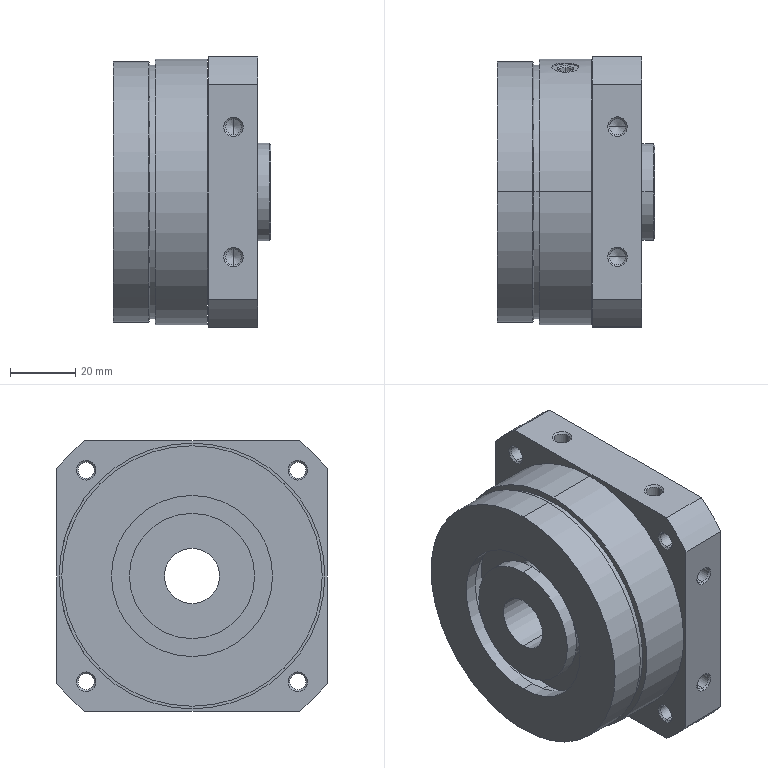Part | STEP file | PN_0043 | 1 solid | 130 faces | box 48.5 x 83 x 83 mm | volume 213563 mm3 | cylinder 56 | cone 52 | plane 20 | spline 2 | commonest cylinder face diameters 4.917 x20 4.134 x4 8.3 x4 106 x4 17 x3 50 x3